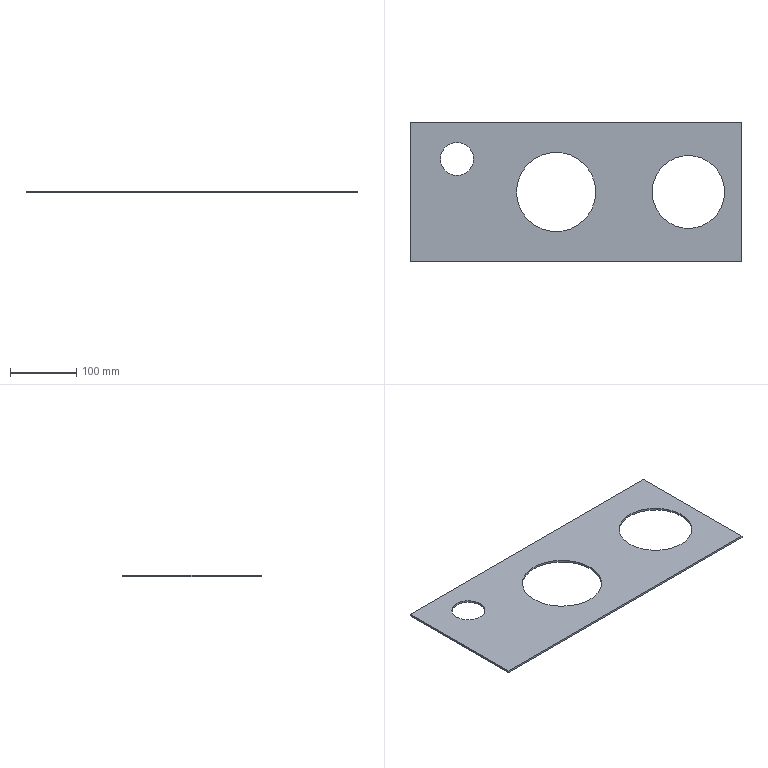Part | SolidWorks | features Cut 1, Extrusion 1 | 1 solid | 12 faces | box 500 x 210 x 3 mm | volume 246670 mm3 | cylinder 6 | plane 6 | commonest cylinder face diameters 50 x2 110 x2 120 x2
STEP:
#1=CARTESIAN_POINT('',(95.,155.,0.));
#2=VERTEX_POINT('',#1);
#3=CARTESIAN_POINT('',(45.,155.,0.));
#4=VERTEX_POINT('',#3);
#5=CARTESIAN_POINT('',(70.,155.,0.));
#6=DIRECTION('',(0.,0.,-1.));
#7=DIRECTION('',(-1.,0.,0.));
#8=AXIS2_PLACEMENT_3D('',#5,#6,#7);
#9=CIRCLE('',#8,25.);
#10=EDGE_CURVE('',#2,#4,#9,.T.);
#11=ORIENTED_EDGE('',*,*,#10,.T.);
#12=CARTESIAN_POINT('',(45.,155.,3.));
#13=VERTEX_POINT('',#12);
#14=CARTESIAN_POINT('',(45.,155.,-7.));
#15=DIRECTION('',(0.,0.,1.));
#16=VECTOR('',#15,1000.);
#17=LINE('',#14,#16);
#18=EDGE_CURVE('',#4,#13,#17,.T.);
#19=ORIENTED_EDGE('',*,*,#18,.T.);
#20=CARTESIAN_POINT('',(95.,155.,3.));
#21=VERTEX_POINT('',#20);
#22=CARTESIAN_POINT('',(70.,155.,3.));
#23=DIRECTION('',(0.,0.,1.));
#24=DIRECTION('',(1.,0.,0.));
#25=AXIS2_PLACEMENT_3D('',#22,#23,#24);
#26=CIRCLE('',#25,25.);
#27=EDGE_CURVE('',#13,#21,#26,.T.);
#28=ORIENTED_EDGE('',*,*,#27,.T.);
#29=CARTESIAN_POINT('',(95.,155.,-7.));
#30=DIRECTION('',(0.,0.,1.));
#31=VECTOR('',#30,1000.);
#32=LINE('',#29,#31);
#33=EDGE_CURVE('',#2,#21,#32,.T.);
#34=ORIENTED_EDGE('',*,*,#33,.F.);
#35=EDGE_LOOP('',(#11,#19,#28,#34));
#36=FACE_OUTER_BOUND('',#35,.T.);
#37=CARTESIAN_POINT('',(70.,155.,-7.));
#38=DIRECTION('',(0.,0.,1.));
#39=DIRECTION('',(1.,0.,0.));
#40=AXIS2_PLACEMENT_3D('',#37,#38,#39);
#41=CYLINDRICAL_SURFACE('',#40,25.);
#42=ADVANCED_FACE('',(#36),#41,.F.);
#43=CARTESIAN_POINT('',(280.,105.,0.));
#44=VERTEX_POINT('',#43);
#45=CARTESIAN_POINT('',(160.,105.,0.));
#46=VERTEX_POINT('',#45);
#47=CARTESIAN_POINT('',(220.,105.,0.));
#48=DIRECTION('',(0.,0.,-1.));
#49=DIRECTION('',(-1.,0.,0.));
#50=AXIS2_PLACEMENT_3D('',#47,#48,#49);
#51=CIRCLE('',#50,60.);
#52=EDGE_CURVE('',#44,#46,#51,.T.);
#53=ORIENTED_EDGE('',*,*,#52,.T.);
#54=CARTESIAN_POINT('',(160.,105.,3.));
#55=VERTEX_POINT('',#54);
#56=CARTESIAN_POINT('',(160.,105.,-7.));
#57=DIRECTION('',(0.,0.,1.));
#58=VECTOR('',#57,1000.);
#59=LINE('',#56,#58);
#60=EDGE_CURVE('',#46,#55,#59,.T.);
#61=ORIENTED_EDGE('',*,*,#60,.T.);
#62=CARTESIAN_POINT('',(280.,105.,3.));
#63=VERTEX_POINT('',#62);
#64=CARTESIAN_POINT('',(220.,105.,3.));
#65=DIRECTION('',(0.,0.,1.));
#66=DIRECTION('',(1.,0.,0.));
#67=AXIS2_PLACEMENT_3D('',#64,#65,#66);
#68=CIRCLE('',#67,60.);
#69=EDGE_CURVE('',#55,#63,#68,.T.);
#70=ORIENTED_EDGE('',*,*,#69,.T.);
#71=CARTESIAN_POINT('',(280.,105.,-7.));
#72=DIRECTION('',(0.,0.,1.));
#73=VECTOR('',#72,1000.);
#74=LINE('',#71,#73);
#75=EDGE_CURVE('',#44,#63,#74,.T.);
#76=ORIENTED_EDGE('',*,*,#75,.F.);
#77=EDGE_LOOP('',(#53,#61,#70,#76));
#78=FACE_OUTER_BOUND('',#77,.T.);
#79=CARTESIAN_POINT('',(220.,105.,-7.));
#80=DIRECTION('',(0.,0.,1.));
#81=DIRECTION('',(1.,0.,0.));
#82=AXIS2_PLACEMENT_3D('',#79,#80,#81);
#83=CYLINDRICAL_SURFACE('',#82,60.);
#84=ADVANCED_FACE('',(#78),#83,.F.);
#85=CARTESIAN_POINT('',(475.,105.,0.));
#86=VERTEX_POINT('',#85);
#87=CARTESIAN_POINT('',(365.,105.,0.));
#88=VERTEX_POINT('',#87);
#89=CARTESIAN_POINT('',(420.,105.,0.));
#90=DIRECTION('',(0.,0.,-1.));
#91=DIRECTION('',(-1.,0.,0.));
#92=AXIS2_PLACEMENT_3D('',#89,#90,#91);
#93=CIRCLE('',#92,55.);
#94=EDGE_CURVE('',#86,#88,#93,.T.);
#95=ORIENTED_EDGE('',*,*,#94,.T.);
#96=CARTESIAN_POINT('',(365.,105.,3.));
#97=VERTEX_POINT('',#96);
#98=CARTESIAN_POINT('',(365.,105.,-7.));
#99=DIRECTION('',(0.,0.,1.));
#100=VECTOR('',#99,1000.);
#101=LINE('',#98,#100);
#102=EDGE_CURVE('',#88,#97,#101,.T.);
#103=ORIENTED_EDGE('',*,*,#102,.T.);
#104=CARTESIAN_POINT('',(475.,105.,3.));
#105=VERTEX_POINT('',#104);
#106=CARTESIAN_POINT('',(420.,105.,3.));
#107=DIRECTION('',(0.,0.,1.));
#108=DIRECTION('',(1.,0.,0.));
#109=AXIS2_PLACEMENT_3D('',#106,#107,#108);
#110=CIRCLE('',#109,55.);
#111=EDGE_CURVE('',#97,#105,#110,.T.);
#112=ORIENTED_EDGE('',*,*,#111,.T.);
#113=CARTESIAN_POINT('',(475.,105.,-7.));
#114=DIRECTION('',(0.,0.,1.));
#115=VECTOR('',#114,1000.);
#116=LINE('',#113,#115);
#117=EDGE_CURVE('',#86,#105,#116,.T.);
#118=ORIENTED_EDGE('',*,*,#117,.F.);
#119=EDGE_LOOP('',(#95,#103,#112,#118));
#120=FACE_OUTER_BOUND('',#119,.T.);
#121=CARTESIAN_POINT('',(420.,105.,-7.));
#122=DIRECTION('',(0.,0.,1.));
#123=DIRECTION('',(1.,0.,0.));
#124=AXIS2_PLACEMENT_3D('',#121,#122,#123);
#125=CYLINDRICAL_SURFACE('',#124,55.);
#126=ADVANCED_FACE('',(#120),#125,.F.);
#127=CARTESIAN_POINT('',(0.,210.,0.));
#128=VERTEX_POINT('',#127);
#129=CARTESIAN_POINT('',(0.,0.,0.));
#130=VERTEX_POINT('',#129);
#131=CARTESIAN_POINT('',(0.,0.,0.));
#132=DIRECTION('',(0.,-1.,0.));
#133=VECTOR('',#132,1000.);
#134=LINE('',#131,#133);
#135=EDGE_CURVE('',#128,#130,#134,.T.);
#136=ORIENTED_EDGE('',*,*,#135,.T.);
#137=CARTESIAN_POINT('',(0.,0.,3.));
#138=VERTEX_POINT('',#137);
#139=CARTESIAN_POINT('',(0.,0.,3.));
#140=DIRECTION('',(0.,0.,-1.));
#141=VECTOR('',#140,1000.);
#142=LINE('',#139,#141);
#143=EDGE_CURVE('',#138,#130,#142,.T.);
#144=ORIENTED_EDGE('',*,*,#143,.F.);
#145=CARTESIAN_POINT('',(0.,210.,3.));
#146=VERTEX_POINT('',#145);
#147=CARTESIAN_POINT('',(0.,0.,3.));
#148=DIRECTION('',(0.,-1.,0.));
#149=VECTOR('',#148,1000.);
#150=LINE('',#147,#149);
#151=EDGE_CURVE('',#146,#138,#150,.T.);
#152=ORIENTED_EDGE('',*,*,#151,.F.);
#153=CARTESIAN_POINT('',(0.,210.,3.));
#154=DIRECTION('',(0.,0.,-1.));
#155=VECTOR('',#154,1000.);
#156=LINE('',#153,#155);
#157=EDGE_CURVE('',#146,#128,#156,.T.);
#158=ORIENTED_EDGE('',*,*,#157,.T.);
#159=EDGE_LOOP('',(#136,#144,#152,#158));
#160=FACE_OUTER_BOUND('',#159,.T.);
#161=CARTESIAN_POINT('',(0.,0.,3.));
#162=DIRECTION('',(1.,0.,0.));
#163=DIRECTION('',(0.,0.,-1.));
#164=AXIS2_PLACEMENT_3D('',#161,#162,#163);
#165=PLANE('',#164);
#166=ADVANCED_FACE('',(#160),#165,.F.);
#167=CARTESIAN_POINT('',(500.,0.,0.));
#168=VERTEX_POINT('',#167);
#169=CARTESIAN_POINT('',(0.,0.,0.));
#170=DIRECTION('',(1.,0.,0.));
#171=VECTOR('',#170,1000.);
#172=LINE('',#169,#171);
#173=EDGE_CURVE('',#130,#168,#172,.T.);
#174=ORIENTED_EDGE('',*,*,#173,.T.);
#175=CARTESIAN_POINT('',(500.,0.,3.));
#176=VERTEX_POINT('',#175);
#177=CARTESIAN_POINT('',(500.,0.,3.));
#178=DIRECTION('',(0.,0.,-1.));
#179=VECTOR('',#178,1000.);
#180=LINE('',#177,#179);
#181=EDGE_CURVE('',#176,#168,#180,.T.);
#182=ORIENTED_EDGE('',*,*,#181,.F.);
#183=CARTESIAN_POINT('',(0.,0.,3.));
#184=DIRECTION('',(1.,0.,0.));
#185=VECTOR('',#184,1000.);
#186=LINE('',#183,#185);
#187=EDGE_CURVE('',#138,#176,#186,.T.);
#188=ORIENTED_EDGE('',*,*,#187,.F.);
#189=ORIENTED_EDGE('',*,*,#143,.T.);
#190=EDGE_LOOP('',(#174,#182,#188,#189));
#191=FACE_OUTER_BOUND('',#190,.T.);
#192=CARTESIAN_POINT('',(0.,0.,3.));
#193=DIRECTION('',(0.,1.,0.));
#194=DIRECTION('',(0.,0.,1.));
#195=AXIS2_PLACEMENT_3D('',#192,#193,#194);
#196=PLANE('',#195);
#197=ADVANCED_FACE('',(#191),#196,.F.);
#198=CARTESIAN_POINT('',(500.,210.,0.));
#199=VERTEX_POINT('',#198);
#200=CARTESIAN_POINT('',(500.,0.,0.));
#201=DIRECTION('',(0.,1.,0.));
#202=VECTOR('',#201,1000.);
#203=LINE('',#200,#202);
#204=EDGE_CURVE('',#168,#199,#203,.T.);
#205=ORIENTED_EDGE('',*,*,#204,.T.);
#206=CARTESIAN_POINT('',(500.,210.,3.));
#207=VERTEX_POINT('',#206);
#208=CARTESIAN_POINT('',(500.,210.,3.));
#209=DIRECTION('',(0.,0.,-1.));
#210=VECTOR('',#209,1000.);
#211=LINE('',#208,#210);
#212=EDGE_CURVE('',#207,#199,#211,.T.);
#213=ORIENTED_EDGE('',*,*,#212,.F.);
#214=CARTESIAN_POINT('',(500.,0.,3.));
#215=DIRECTION('',(0.,1.,0.));
#216=VECTOR('',#215,1000.);
#217=LINE('',#214,#216);
#218=EDGE_CURVE('',#176,#207,#217,.T.);
#219=ORIENTED_EDGE('',*,*,#218,.F.);
#220=ORIENTED_EDGE('',*,*,#181,.T.);
#221=EDGE_LOOP('',(#205,#213,#219,#220));
#222=FACE_OUTER_BOUND('',#221,.T.);
#223=CARTESIAN_POINT('',(500.,0.,3.));
#224=DIRECTION('',(-1.,0.,0.));
#225=DIRECTION('',(0.,0.,1.));
#226=AXIS2_PLACEMENT_3D('',#223,#224,#225);
#227=PLANE('',#226);
#228=ADVANCED_FACE('',(#222),#227,.F.);
#229=CARTESIAN_POINT('',(0.,210.,0.));
#230=DIRECTION('',(-1.,0.,0.));
#231=VECTOR('',#230,1000.);
#232=LINE('',#229,#231);
#233=EDGE_CURVE('',#199,#128,#232,.T.);
#234=ORIENTED_EDGE('',*,*,#233,.T.);
#235=ORIENTED_EDGE('',*,*,#157,.F.);
#236=CARTESIAN_POINT('',(0.,210.,3.));
#237=DIRECTION('',(-1.,0.,0.));
#238=VECTOR('',#237,1000.);
#239=LINE('',#236,#238);
#240=EDGE_CURVE('',#207,#146,#239,.T.);
#241=ORIENTED_EDGE('',*,*,#240,.F.);
#242=ORIENTED_EDGE('',*,*,#212,.T.);
#243=EDGE_LOOP('',(#234,#235,#241,#242));
#244=FACE_OUTER_BOUND('',#243,.T.);
#245=CARTESIAN_POINT('',(0.,210.,3.));
#246=DIRECTION('',(0.,-1.,0.));
#247=DIRECTION('',(0.,0.,-1.));
#248=AXIS2_PLACEMENT_3D('',#245,#246,#247);
#249=PLANE('',#248);
#250=ADVANCED_FACE('',(#244),#249,.F.);
#251=CARTESIAN_POINT('',(70.,155.,3.));
#252=DIRECTION('',(0.,0.,1.));
#253=DIRECTION('',(1.,0.,0.));
#254=AXIS2_PLACEMENT_3D('',#251,#252,#253);
#255=CIRCLE('',#254,25.);
#256=EDGE_CURVE('',#21,#13,#255,.T.);
#257=ORIENTED_EDGE('',*,*,#256,.F.);
#258=ORIENTED_EDGE('',*,*,#27,.F.);
#259=EDGE_LOOP('',(#257,#258));
#260=FACE_BOUND('',#259,.T.);
#261=CARTESIAN_POINT('',(220.,105.,3.));
#262=DIRECTION('',(0.,0.,1.));
#263=DIRECTION('',(1.,0.,0.));
#264=AXIS2_PLACEMENT_3D('',#261,#262,#263);
#265=CIRCLE('',#264,60.);
#266=EDGE_CURVE('',#63,#55,#265,.T.);
#267=ORIENTED_EDGE('',*,*,#266,.F.);
#268=ORIENTED_EDGE('',*,*,#69,.F.);
#269=EDGE_LOOP('',(#267,#268));
#270=FACE_BOUND('',#269,.T.);
#271=CARTESIAN_POINT('',(420.,105.,3.));
#272=DIRECTION('',(0.,0.,1.));
#273=DIRECTION('',(1.,0.,0.));
#274=AXIS2_PLACEMENT_3D('',#271,#272,#273);
#275=CIRCLE('',#274,55.);
#276=EDGE_CURVE('',#105,#97,#275,.T.);
#277=ORIENTED_EDGE('',*,*,#276,.F.);
#278=ORIENTED_EDGE('',*,*,#111,.F.);
#279=EDGE_LOOP('',(#277,#278));
#280=FACE_BOUND('',#279,.T.);
#281=ORIENTED_EDGE('',*,*,#151,.T.);
#282=ORIENTED_EDGE('',*,*,#187,.T.);
#283=ORIENTED_EDGE('',*,*,#218,.T.);
#284=ORIENTED_EDGE('',*,*,#240,.T.);
#285=EDGE_LOOP('',(#281,#282,#283,#284));
#286=FACE_OUTER_BOUND('',#285,.T.);
#287=CARTESIAN_POINT('',(0.,0.,3.));
#288=DIRECTION('',(0.,0.,-1.));
#289=DIRECTION('',(-1.,0.,0.));
#290=AXIS2_PLACEMENT_3D('',#287,#288,#289);
#291=PLANE('',#290);
#292=ADVANCED_FACE('',(#260,#270,#280,#286),#291,.F.);
#293=ORIENTED_EDGE('',*,*,#10,.F.);
#294=CARTESIAN_POINT('',(70.,155.,0.));
#295=DIRECTION('',(0.,0.,-1.));
#296=DIRECTION('',(-1.,0.,0.));
#297=AXIS2_PLACEMENT_3D('',#294,#295,#296);
#298=CIRCLE('',#297,25.);
#299=EDGE_CURVE('',#4,#2,#298,.T.);
#300=ORIENTED_EDGE('',*,*,#299,.F.);
#301=EDGE_LOOP('',(#293,#300));
#302=FACE_BOUND('',#301,.T.);
#303=ORIENTED_EDGE('',*,*,#52,.F.);
#304=CARTESIAN_POINT('',(220.,105.,0.));
#305=DIRECTION('',(0.,0.,-1.));
#306=DIRECTION('',(-1.,0.,0.));
#307=AXIS2_PLACEMENT_3D('',#304,#305,#306);
#308=CIRCLE('',#307,60.);
#309=EDGE_CURVE('',#46,#44,#308,.T.);
#310=ORIENTED_EDGE('',*,*,#309,.F.);
#311=EDGE_LOOP('',(#303,#310));
#312=FACE_BOUND('',#311,.T.);
#313=ORIENTED_EDGE('',*,*,#94,.F.);
#314=CARTESIAN_POINT('',(420.,105.,0.));
#315=DIRECTION('',(0.,0.,-1.));
#316=DIRECTION('',(-1.,0.,0.));
#317=AXIS2_PLACEMENT_3D('',#314,#315,#316);
#318=CIRCLE('',#317,55.);
#319=EDGE_CURVE('',#88,#86,#318,.T.);
#320=ORIENTED_EDGE('',*,*,#319,.F.);
#321=EDGE_LOOP('',(#313,#320));
#322=FACE_BOUND('',#321,.T.);
#323=ORIENTED_EDGE('',*,*,#135,.F.);
#324=ORIENTED_EDGE('',*,*,#233,.F.);
#325=ORIENTED_EDGE('',*,*,#204,.F.);
#326=ORIENTED_EDGE('',*,*,#173,.F.);
#327=EDGE_LOOP('',(#323,#324,#325,#326));
#328=FACE_OUTER_BOUND('',#327,.T.);
#329=CARTESIAN_POINT('',(0.,0.,0.));
#330=DIRECTION('',(0.,0.,-1.));
#331=DIRECTION('',(-1.,0.,0.));
#332=AXIS2_PLACEMENT_3D('',#329,#330,#331);
#333=PLANE('',#332);
#334=ADVANCED_FACE('',(#302,#312,#322,#328),#333,.T.);
#335=ORIENTED_EDGE('',*,*,#102,.F.);
#336=ORIENTED_EDGE('',*,*,#319,.T.);
#337=ORIENTED_EDGE('',*,*,#117,.T.);
#338=ORIENTED_EDGE('',*,*,#276,.T.);
#339=EDGE_LOOP('',(#335,#336,#337,#338));
#340=FACE_OUTER_BOUND('',#339,.T.);
#341=CARTESIAN_POINT('',(420.,105.,-7.));
#342=DIRECTION('',(0.,0.,1.));
#343=DIRECTION('',(1.,0.,0.));
#344=AXIS2_PLACEMENT_3D('',#341,#342,#343);
#345=CYLINDRICAL_SURFACE('',#344,55.);
#346=ADVANCED_FACE('',(#340),#345,.F.);
#347=ORIENTED_EDGE('',*,*,#60,.F.);
#348=ORIENTED_EDGE('',*,*,#309,.T.);
#349=ORIENTED_EDGE('',*,*,#75,.T.);
#350=ORIENTED_EDGE('',*,*,#266,.T.);
#351=EDGE_LOOP('',(#347,#348,#349,#350));
#352=FACE_OUTER_BOUND('',#351,.T.);
#353=CARTESIAN_POINT('',(220.,105.,-7.));
#354=DIRECTION('',(0.,0.,1.));
#355=DIRECTION('',(1.,0.,0.));
#356=AXIS2_PLACEMENT_3D('',#353,#354,#355);
#357=CYLINDRICAL_SURFACE('',#356,60.);
#358=ADVANCED_FACE('',(#352),#357,.F.);
#359=ORIENTED_EDGE('',*,*,#18,.F.);
#360=ORIENTED_EDGE('',*,*,#299,.T.);
#361=ORIENTED_EDGE('',*,*,#33,.T.);
#362=ORIENTED_EDGE('',*,*,#256,.T.);
#363=EDGE_LOOP('',(#359,#360,#361,#362));
#364=FACE_OUTER_BOUND('',#363,.T.);
#365=CARTESIAN_POINT('',(70.,155.,-7.));
#366=DIRECTION('',(0.,0.,1.));
#367=DIRECTION('',(1.,0.,0.));
#368=AXIS2_PLACEMENT_3D('',#365,#366,#367);
#369=CYLINDRICAL_SURFACE('',#368,25.);
#370=ADVANCED_FACE('',(#364),#369,.F.);
#371=CLOSED_SHELL('',(#42,#84,#126,#166,#197,#228,#250,#292,#334,#346,#358,#370));
#372=MANIFOLD_SOLID_BREP('',#371);
#373=CARTESIAN_POINT('',(0.,0.,0.));
#374=DIRECTION('',(0.,0.,1.));
#375=DIRECTION('',(1.,0.,0.));
#376=AXIS2_PLACEMENT_3D('',#373,#374,#375);
#377=(LENGTH_UNIT()NAMED_UNIT(*)SI_UNIT(.MILLI.,.METRE.));
#378=UNCERTAINTY_MEASURE_WITH_UNIT(LENGTH_MEASURE(0.00001),#377,'','');
#379=(NAMED_UNIT(*)PLANE_ANGLE_UNIT()SI_UNIT($,.RADIAN.));
#380=(NAMED_UNIT(*)SI_UNIT($,.STERADIAN.)SOLID_ANGLE_UNIT());
#381=(GEOMETRIC_REPRESENTATION_CONTEXT(3)GLOBAL_UNCERTAINTY_ASSIGNED_CONTEXT((#378))GLOBAL_UNIT_ASSIGNED_CONTEXT((#377,#379,#380))REPRESENTATION_CONTEXT('',''));
#382=ADVANCED_BREP_SHAPE_REPRESENTATION('',(#372,#376),#381);